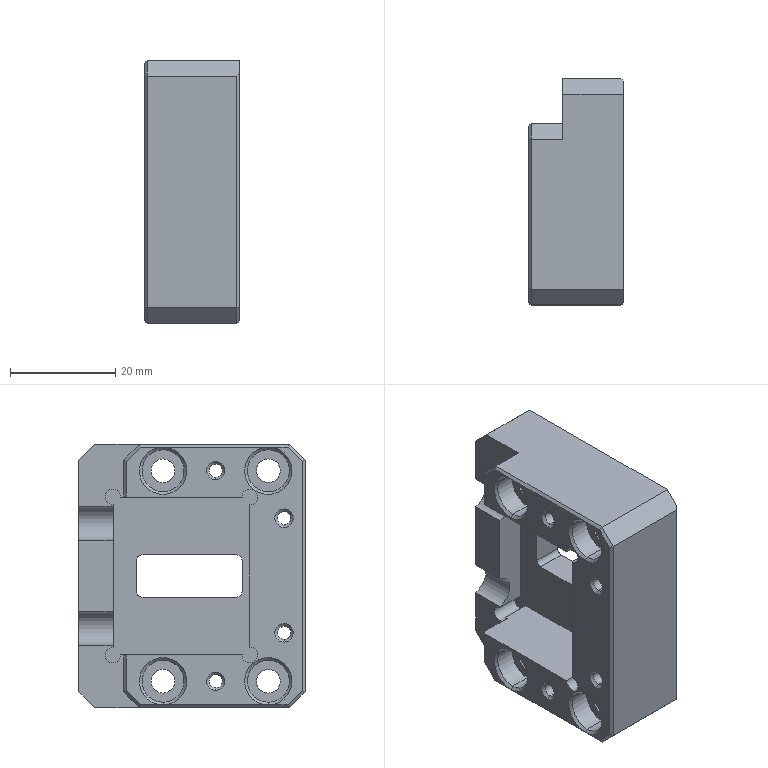Part | SolidWorks | features Chamfer 5, Cut 3, HoleWzd 3, 3DProfileFeature 1, Extrusion 1 | 1 solid | 130 faces | box 18 x 43 x 50 mm | volume 22818 mm3 | plane 50 | cylinder 44 | cone 36 | commonest cylinder face diameters 2.5 x8 4.5 x8 8 x8 3 x6 2 x4 4 x4